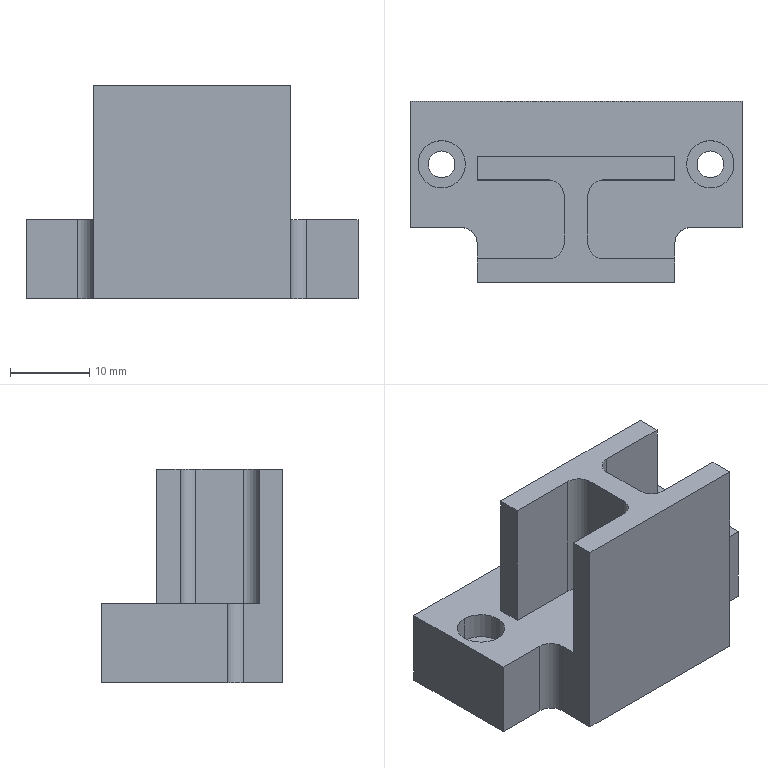CAM job | NX | 3-axis milling | part box 42 x 23 x 27 mm | stock box 48 x 29 x 28 mm
Tools:
number,name,description,diameter,corner_radius,flute_length,length,flutes
1,D50,Milling Tool-5 Parameters,50.0,0.0,50.0,75.0,2
3,D10,Milling Tool-5 Parameters,10.0,0.0,50.0,75.0,2
4,D10JING,Milling Tool-5 Parameters,10.0,0.0,50.0,75.0,2
10,D4,Milling Tool-5 Parameters,4.0,0.0,50.0,75.0,2
8,D6,Milling Tool-5 Parameters,6.0,0.0,50.0,75.0,2
2,D6A45,Milling Tool-5 Parameters,6.0,0.0,3.0,3.0,2
Operations:
program,operation,operation_type,tool,method,geometry_group,spindle_rpm,surface_speed,feed_per_tooth,feed_cut,feed_plunge,cut_length_mm,path_length_mm,cut_time_min,machine_time_min
1-45-30-25毛胚,FLOOR_WALL,VolumeBased25DMillingOperation,D50,METHOD,A,6500.0,1286.0,0.0962,1250.0,100.0,110.0,164.0,0.088,0.0934
1-45-30-25毛胚,ADAPTIVE_MILLING,CavityMilling,D10,METHOD,A,7000.0,219.0,0.2143,3000.0,1000.0,4353.43,4719.195,1.457,1.494
1-45-30-25毛胚,ZLEVEL_PROFILE_COPY_COPY_1_COPY_COPY_COPY_1,ZLevelMilling,D10JING,METHOD,A,7000.0,219.0,0.0714,1000.0,100.0,160.258,274.258,0.1603,0.1717
1-45-30-25毛胚,ZLEVEL_PROFILE_COPY_COPY_1_COPY_COPY_COPY_1_COPY_COPY_1_COPY,ZLevelMilling,D6,METHOD,A,7000.0,131.0,0.1071,1500.0,100.0,2288.239,3135.088,1.526,1.61
1-45-30-25毛胚,ZLEVEL_PROFILE_COPY_COPY_1_COPY_COPY_COPY_1_COPY_COPY_1,ZLevelMilling,D4,METHOD,A,7000.0,131.0,0.1071,1500.0,100.0,873.064,1887.893,0.582,0.6835
1-45-30-25毛胚,FLOOR_WALL_1_COPY_1_COPY,VolumeBased25DMillingOperation,D4,METHOD,A,7000.0,87.0,0.0714,1000.0,100.0,211.66,407.844,0.2117,0.2313
1-45-30-25毛胚,FLOOR_WALL_1_COPY_1,VolumeBased25DMillingOperation,D4,METHOD,A,7000.0,87.0,0.0714,1000.0,100.0,556.797,885.694,0.5568,0.5897
1-45-30-25毛胚,HOLE_MILLING,CylinderMilling,D4,METHOD,A,7000.0,131.0,0.1071,1500.0,100.0,182.399,410.199,0.1216,0.1444
1-45-30-25毛胚,ZLEVEL_PROFILE_COPY_1_COPY_COPY_COPY_COPY_2_COPY,ZLevelMilling,D6A45,METHOD,A,7000.0,131.0,0.0714,1000.0,1000.0,131.691,193.691,0.1317,0.1379
1-45-30-25毛胚,ZLEVEL_PROFILE_COPY_1_COPY_COPY_COPY_COPY_2_COPY_COPY,ZLevelMilling,D6A45,METHOD,A,7000.0,131.0,0.0714,1000.0,1000.0,122.464,481.594,0.1225,0.1584